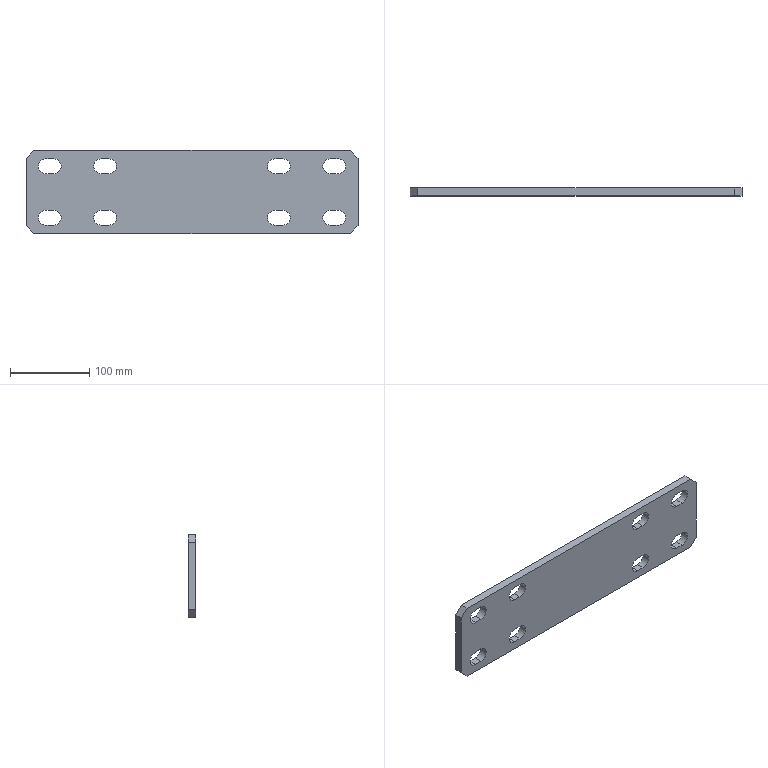Part | STEP file | E3-导轨连接Plate 2 | 1 solid | 42 faces | box 420 x 10 x 105 mm | volume 401118 mm3 | plane 26 | cylinder 16 | commonest cylinder face diameters 19 x16